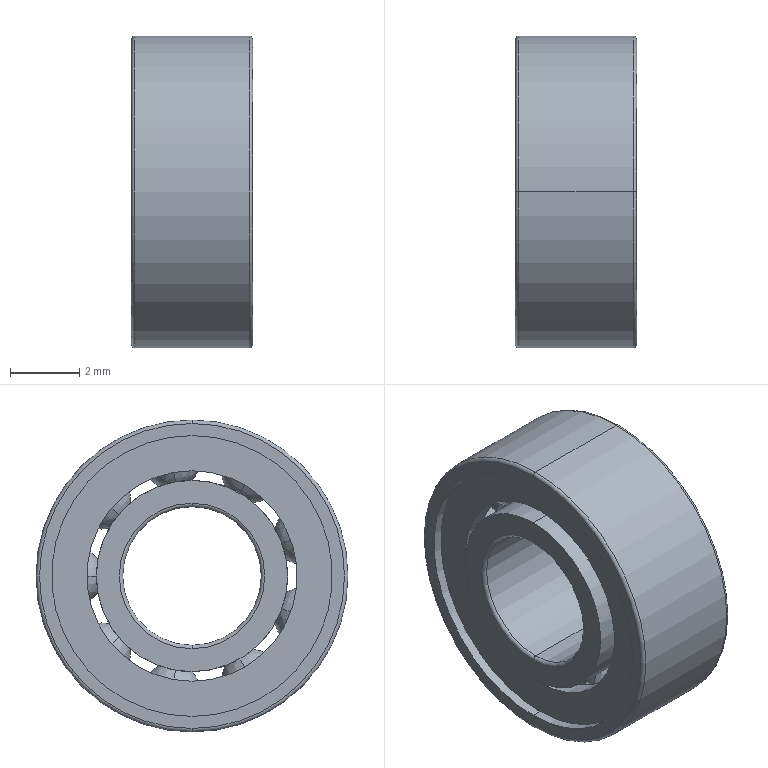Part | NX | features BREP 1 | 1 solid | 160 faces | box 3.5 x 9 x 9 mm | volume 125.696 mm3 | sphere 72 | torus 38 | plane 26 | cylinder 24 | commonest cylinder face diameters 8.1 x8 5.52 x4 6.074 x4 4 x2 6.348 x2 7.272 x2